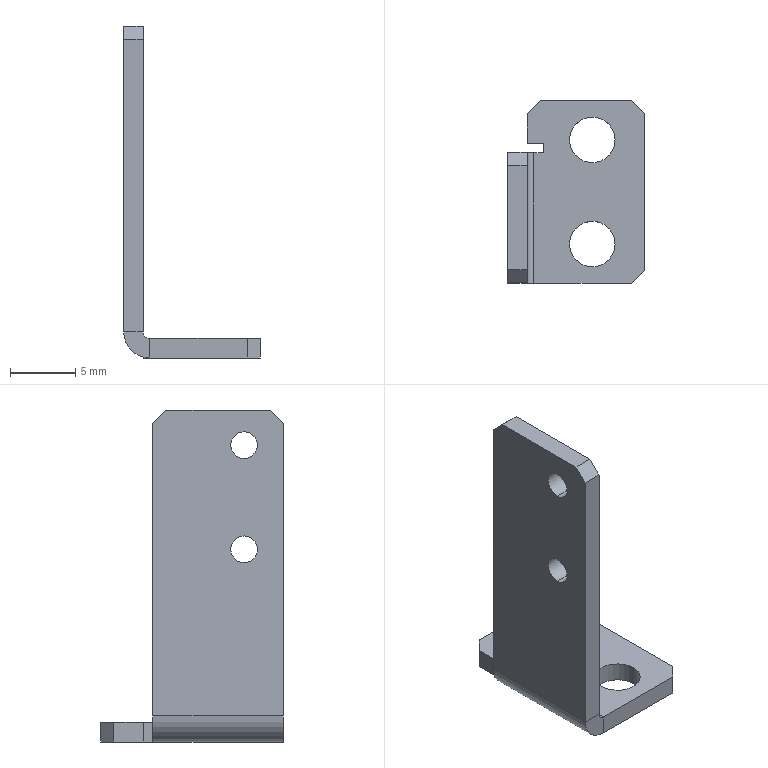Part | SolidWorks | features HoleWzd 2, Chamfer 1, EdgeFlange 1, FlatPattern 1, SMBaseFlange 1, SheetMetal 1 | 1 solid | 31 faces | box 10.5 x 14 x 25.5 mm | volume 519.531 mm3 | plane 21 | cylinder 10 | commonest cylinder face diameters 2.05 x4 3.5 x4 1 x1 4 x1
STEP:
#1=CARTESIAN_POINT('',(-1.25,-4.,-1.5));
#2=VERTEX_POINT('',#1);
#3=CARTESIAN_POINT('',(2.25,-4.,-1.5));
#4=VERTEX_POINT('',#3);
#5=CARTESIAN_POINT('',(0.5,-4.,-1.5));
#6=DIRECTION('',(0.,0.,1.));
#7=DIRECTION('',(1.,0.,0.));
#8=AXIS2_PLACEMENT_3D('',#5,#6,#7);
#9=CIRCLE('',#8,1.75);
#10=EDGE_CURVE('',#2,#4,#9,.T.);
#11=ORIENTED_EDGE('',*,*,#10,.F.);
#12=CARTESIAN_POINT('',(-1.25,-4.,0.));
#13=VERTEX_POINT('',#12);
#14=CARTESIAN_POINT('',(-1.25,-4.,0.));
#15=DIRECTION('',(0.,0.,1.));
#16=VECTOR('',#15,1000.);
#17=LINE('',#14,#16);
#18=EDGE_CURVE('',#2,#13,#17,.T.);
#19=ORIENTED_EDGE('',*,*,#18,.T.);
#20=CARTESIAN_POINT('',(2.25,-4.,0.));
#21=VERTEX_POINT('',#20);
#22=CARTESIAN_POINT('',(0.5,-4.,0.));
#23=DIRECTION('',(0.,0.,1.));
#24=DIRECTION('',(1.,0.,0.));
#25=AXIS2_PLACEMENT_3D('',#22,#23,#24);
#26=CIRCLE('',#25,1.75);
#27=EDGE_CURVE('',#13,#21,#26,.T.);
#28=ORIENTED_EDGE('',*,*,#27,.T.);
#29=CARTESIAN_POINT('',(2.25,-4.,0.));
#30=DIRECTION('',(0.,0.,1.));
#31=VECTOR('',#30,1000.);
#32=LINE('',#29,#31);
#33=EDGE_CURVE('',#4,#21,#32,.T.);
#34=ORIENTED_EDGE('',*,*,#33,.F.);
#35=EDGE_LOOP('',(#11,#19,#28,#34));
#36=FACE_OUTER_BOUND('',#35,.T.);
#37=CARTESIAN_POINT('',(0.5,-4.,0.));
#38=DIRECTION('',(0.,0.,1.));
#39=DIRECTION('',(1.,0.,0.));
#40=AXIS2_PLACEMENT_3D('',#37,#38,#39);
#41=CYLINDRICAL_SURFACE('',#40,1.75);
#42=ADVANCED_FACE('',(#36),#41,.F.);
#43=CARTESIAN_POINT('',(-1.25,4.,-1.5));
#44=VERTEX_POINT('',#43);
#45=CARTESIAN_POINT('',(2.25,4.,-1.5));
#46=VERTEX_POINT('',#45);
#47=CARTESIAN_POINT('',(0.5,4.,-1.5));
#48=DIRECTION('',(0.,0.,1.));
#49=DIRECTION('',(1.,0.,0.));
#50=AXIS2_PLACEMENT_3D('',#47,#48,#49);
#51=CIRCLE('',#50,1.75);
#52=EDGE_CURVE('',#44,#46,#51,.T.);
#53=ORIENTED_EDGE('',*,*,#52,.F.);
#54=CARTESIAN_POINT('',(-1.25,4.,0.));
#55=VERTEX_POINT('',#54);
#56=CARTESIAN_POINT('',(-1.25,4.,0.));
#57=DIRECTION('',(0.,0.,1.));
#58=VECTOR('',#57,1000.);
#59=LINE('',#56,#58);
#60=EDGE_CURVE('',#44,#55,#59,.T.);
#61=ORIENTED_EDGE('',*,*,#60,.T.);
#62=CARTESIAN_POINT('',(2.25,4.,0.));
#63=VERTEX_POINT('',#62);
#64=CARTESIAN_POINT('',(0.5,4.,0.));
#65=DIRECTION('',(0.,0.,1.));
#66=DIRECTION('',(1.,0.,0.));
#67=AXIS2_PLACEMENT_3D('',#64,#65,#66);
#68=CIRCLE('',#67,1.75);
#69=EDGE_CURVE('',#55,#63,#68,.T.);
#70=ORIENTED_EDGE('',*,*,#69,.T.);
#71=CARTESIAN_POINT('',(2.25,4.,0.));
#72=DIRECTION('',(0.,0.,1.));
#73=VECTOR('',#72,1000.);
#74=LINE('',#71,#73);
#75=EDGE_CURVE('',#46,#63,#74,.T.);
#76=ORIENTED_EDGE('',*,*,#75,.F.);
#77=EDGE_LOOP('',(#53,#61,#70,#76));
#78=FACE_OUTER_BOUND('',#77,.T.);
#79=CARTESIAN_POINT('',(0.5,4.,0.));
#80=DIRECTION('',(0.,0.,1.));
#81=DIRECTION('',(1.,0.,0.));
#82=AXIS2_PLACEMENT_3D('',#79,#80,#81);
#83=CYLINDRICAL_SURFACE('',#82,1.75);
#84=ADVANCED_FACE('',(#78),#83,.F.);
#85=CARTESIAN_POINT('',(-4.5,-4.,14.325));
#86=VERTEX_POINT('',#85);
#87=CARTESIAN_POINT('',(-4.5,-4.,12.275));
#88=VERTEX_POINT('',#87);
#89=CARTESIAN_POINT('',(-4.5,-4.,13.3));
#90=DIRECTION('',(1.,0.,0.));
#91=DIRECTION('',(0.,0.,-1.));
#92=AXIS2_PLACEMENT_3D('',#89,#90,#91);
#93=CIRCLE('',#92,1.025);
#94=EDGE_CURVE('',#86,#88,#93,.T.);
#95=ORIENTED_EDGE('',*,*,#94,.T.);
#96=CARTESIAN_POINT('',(-6.,-4.,12.275));
#97=VERTEX_POINT('',#96);
#98=CARTESIAN_POINT('',(-6.,-4.,12.275));
#99=DIRECTION('',(-1.,0.,0.));
#100=VECTOR('',#99,1000.);
#101=LINE('',#98,#100);
#102=EDGE_CURVE('',#88,#97,#101,.T.);
#103=ORIENTED_EDGE('',*,*,#102,.T.);
#104=CARTESIAN_POINT('',(-6.,-4.,14.325));
#105=VERTEX_POINT('',#104);
#106=CARTESIAN_POINT('',(-6.,-4.,13.3));
#107=DIRECTION('',(-1.,0.,0.));
#108=DIRECTION('',(0.,0.,1.));
#109=AXIS2_PLACEMENT_3D('',#106,#107,#108);
#110=CIRCLE('',#109,1.025);
#111=EDGE_CURVE('',#97,#105,#110,.T.);
#112=ORIENTED_EDGE('',*,*,#111,.T.);
#113=CARTESIAN_POINT('',(-6.,-4.,14.325));
#114=DIRECTION('',(-1.,0.,0.));
#115=VECTOR('',#114,1000.);
#116=LINE('',#113,#115);
#117=EDGE_CURVE('',#86,#105,#116,.T.);
#118=ORIENTED_EDGE('',*,*,#117,.F.);
#119=EDGE_LOOP('',(#95,#103,#112,#118));
#120=FACE_OUTER_BOUND('',#119,.T.);
#121=CARTESIAN_POINT('',(-6.,-4.,13.3));
#122=DIRECTION('',(-1.,0.,0.));
#123=DIRECTION('',(0.,0.,1.));
#124=AXIS2_PLACEMENT_3D('',#121,#122,#123);
#125=CYLINDRICAL_SURFACE('',#124,1.025);
#126=ADVANCED_FACE('',(#120),#125,.F.);
#127=CARTESIAN_POINT('',(-4.5,-4.,22.325));
#128=VERTEX_POINT('',#127);
#129=CARTESIAN_POINT('',(-4.5,-4.,20.275));
#130=VERTEX_POINT('',#129);
#131=CARTESIAN_POINT('',(-4.5,-4.,21.3));
#132=DIRECTION('',(1.,0.,0.));
#133=DIRECTION('',(0.,0.,-1.));
#134=AXIS2_PLACEMENT_3D('',#131,#132,#133);
#135=CIRCLE('',#134,1.025);
#136=EDGE_CURVE('',#128,#130,#135,.T.);
#137=ORIENTED_EDGE('',*,*,#136,.T.);
#138=CARTESIAN_POINT('',(-6.,-4.,20.275));
#139=VERTEX_POINT('',#138);
#140=CARTESIAN_POINT('',(-6.,-4.,20.275));
#141=DIRECTION('',(-1.,0.,0.));
#142=VECTOR('',#141,1000.);
#143=LINE('',#140,#142);
#144=EDGE_CURVE('',#130,#139,#143,.T.);
#145=ORIENTED_EDGE('',*,*,#144,.T.);
#146=CARTESIAN_POINT('',(-6.,-4.,22.325));
#147=VERTEX_POINT('',#146);
#148=CARTESIAN_POINT('',(-6.,-4.,21.3));
#149=DIRECTION('',(-1.,0.,0.));
#150=DIRECTION('',(0.,0.,1.));
#151=AXIS2_PLACEMENT_3D('',#148,#149,#150);
#152=CIRCLE('',#151,1.025);
#153=EDGE_CURVE('',#139,#147,#152,.T.);
#154=ORIENTED_EDGE('',*,*,#153,.T.);
#155=CARTESIAN_POINT('',(-6.,-4.,22.325));
#156=DIRECTION('',(-1.,0.,0.));
#157=VECTOR('',#156,1000.);
#158=LINE('',#155,#157);
#159=EDGE_CURVE('',#128,#147,#158,.T.);
#160=ORIENTED_EDGE('',*,*,#159,.F.);
#161=EDGE_LOOP('',(#137,#145,#154,#160));
#162=FACE_OUTER_BOUND('',#161,.T.);
#163=CARTESIAN_POINT('',(-6.,-4.,21.3));
#164=DIRECTION('',(-1.,0.,0.));
#165=DIRECTION('',(0.,0.,1.));
#166=AXIS2_PLACEMENT_3D('',#163,#164,#165);
#167=CYLINDRICAL_SURFACE('',#166,1.025);
#168=ADVANCED_FACE('',(#162),#167,.F.);
#169=CARTESIAN_POINT('',(-4.,-7.,-1.5));
#170=VERTEX_POINT('',#169);
#171=CARTESIAN_POINT('',(3.5,-7.,-1.5));
#172=VERTEX_POINT('',#171);
#173=CARTESIAN_POINT('',(-4.5,-7.,-1.5));
#174=DIRECTION('',(1.,0.,0.));
#175=VECTOR('',#174,1000.);
#176=LINE('',#173,#175);
#177=EDGE_CURVE('',#170,#172,#176,.T.);
#178=ORIENTED_EDGE('',*,*,#177,.T.);
#179=CARTESIAN_POINT('',(3.5,-7.,0.));
#180=VERTEX_POINT('',#179);
#181=CARTESIAN_POINT('',(3.5,-7.,-1.5));
#182=DIRECTION('',(0.,0.,1.));
#183=VECTOR('',#182,1000.);
#184=LINE('',#181,#183);
#185=EDGE_CURVE('',#172,#180,#184,.T.);
#186=ORIENTED_EDGE('',*,*,#185,.T.);
#187=CARTESIAN_POINT('',(-4.,-7.,0.));
#188=VERTEX_POINT('',#187);
#189=CARTESIAN_POINT('',(-4.5,-7.,0.));
#190=DIRECTION('',(1.,0.,0.));
#191=VECTOR('',#190,1000.);
#192=LINE('',#189,#191);
#193=EDGE_CURVE('',#188,#180,#192,.T.);
#194=ORIENTED_EDGE('',*,*,#193,.F.);
#195=CARTESIAN_POINT('',(-4.,-7.,0.));
#196=DIRECTION('',(0.,0.,-1.));
#197=VECTOR('',#196,1000.);
#198=LINE('',#195,#197);
#199=EDGE_CURVE('',#188,#170,#198,.T.);
#200=ORIENTED_EDGE('',*,*,#199,.T.);
#201=EDGE_LOOP('',(#178,#186,#194,#200));
#202=FACE_OUTER_BOUND('',#201,.T.);
#203=CARTESIAN_POINT('',(-4.5,-7.,-1.5));
#204=DIRECTION('',(0.,-1.,0.));
#205=DIRECTION('',(0.,0.,-1.));
#206=AXIS2_PLACEMENT_3D('',#203,#204,#205);
#207=PLANE('',#206);
#208=ADVANCED_FACE('',(#202),#207,.T.);
#209=CARTESIAN_POINT('',(-4.5,6.,0.));
#210=VERTEX_POINT('',#209);
#211=CARTESIAN_POINT('',(-4.5,3.75,0.));
#212=VERTEX_POINT('',#211);
#213=CARTESIAN_POINT('',(-4.5,7.,0.));
#214=DIRECTION('',(0.,-1.,0.));
#215=VECTOR('',#214,1000.);
#216=LINE('',#213,#215);
#217=EDGE_CURVE('',#210,#212,#216,.T.);
#218=ORIENTED_EDGE('',*,*,#217,.F.);
#219=CARTESIAN_POINT('',(-4.5,6.,-1.5));
#220=VERTEX_POINT('',#219);
#221=CARTESIAN_POINT('',(-4.5,6.,-1.5));
#222=DIRECTION('',(0.,0.,-1.));
#223=VECTOR('',#222,1000.);
#224=LINE('',#221,#223);
#225=EDGE_CURVE('',#210,#220,#224,.T.);
#226=ORIENTED_EDGE('',*,*,#225,.T.);
#227=CARTESIAN_POINT('',(-4.5,3.75,-1.5));
#228=VERTEX_POINT('',#227);
#229=CARTESIAN_POINT('',(-4.5,7.,-1.5));
#230=DIRECTION('',(0.,-1.,0.));
#231=VECTOR('',#230,1000.);
#232=LINE('',#229,#231);
#233=EDGE_CURVE('',#220,#228,#232,.T.);
#234=ORIENTED_EDGE('',*,*,#233,.T.);
#235=CARTESIAN_POINT('',(-4.5,3.75,0.));
#236=DIRECTION('',(0.,0.,-1.));
#237=VECTOR('',#236,1000.);
#238=LINE('',#235,#237);
#239=EDGE_CURVE('',#212,#228,#238,.T.);
#240=ORIENTED_EDGE('',*,*,#239,.F.);
#241=EDGE_LOOP('',(#218,#226,#234,#240));
#242=FACE_OUTER_BOUND('',#241,.T.);
#243=CARTESIAN_POINT('',(-4.5,7.,-1.5));
#244=DIRECTION('',(-1.,0.,0.));
#245=DIRECTION('',(0.,-1.,0.));
#246=AXIS2_PLACEMENT_3D('',#243,#244,#245);
#247=PLANE('',#246);
#248=ADVANCED_FACE('',(#242),#247,.T.);
#249=CARTESIAN_POINT('',(0.5,-4.,-1.5));
#250=DIRECTION('',(0.,0.,1.));
#251=DIRECTION('',(1.,0.,0.));
#252=AXIS2_PLACEMENT_3D('',#249,#250,#251);
#253=CIRCLE('',#252,1.75);
#254=EDGE_CURVE('',#4,#2,#253,.T.);
#255=ORIENTED_EDGE('',*,*,#254,.T.);
#256=ORIENTED_EDGE('',*,*,#10,.T.);
#257=EDGE_LOOP('',(#255,#256));
#258=FACE_BOUND('',#257,.T.);
#259=CARTESIAN_POINT('',(0.5,4.,-1.5));
#260=DIRECTION('',(0.,0.,1.));
#261=DIRECTION('',(1.,0.,0.));
#262=AXIS2_PLACEMENT_3D('',#259,#260,#261);
#263=CIRCLE('',#262,1.75);
#264=EDGE_CURVE('',#46,#44,#263,.T.);
#265=ORIENTED_EDGE('',*,*,#264,.T.);
#266=ORIENTED_EDGE('',*,*,#52,.T.);
#267=EDGE_LOOP('',(#265,#266));
#268=FACE_BOUND('',#267,.T.);
#269=ORIENTED_EDGE('',*,*,#233,.F.);
#270=CARTESIAN_POINT('',(-3.5,7.,-1.5));
#271=VERTEX_POINT('',#270);
#272=CARTESIAN_POINT('',(-3.5,7.,-1.5));
#273=DIRECTION('',(0.7071,0.7071,0.));
#274=VECTOR('',#273,1000.);
#275=LINE('',#272,#274);
#276=EDGE_CURVE('',#220,#271,#275,.T.);
#277=ORIENTED_EDGE('',*,*,#276,.T.);
#278=CARTESIAN_POINT('',(3.5,7.,-1.5));
#279=VERTEX_POINT('',#278);
#280=CARTESIAN_POINT('',(-4.5,7.,-1.5));
#281=DIRECTION('',(-1.,0.,0.));
#282=VECTOR('',#281,1000.);
#283=LINE('',#280,#282);
#284=EDGE_CURVE('',#279,#271,#283,.T.);
#285=ORIENTED_EDGE('',*,*,#284,.F.);
#286=CARTESIAN_POINT('',(4.5,6.,-1.5));
#287=VERTEX_POINT('',#286);
#288=CARTESIAN_POINT('',(4.5,6.,-1.5));
#289=DIRECTION('',(0.7071,-0.7071,0.));
#290=VECTOR('',#289,1000.);
#291=LINE('',#288,#290);
#292=EDGE_CURVE('',#279,#287,#291,.T.);
#293=ORIENTED_EDGE('',*,*,#292,.T.);
#294=CARTESIAN_POINT('',(4.5,-6.,-1.5));
#295=VERTEX_POINT('',#294);
#296=CARTESIAN_POINT('',(4.5,7.,-1.5));
#297=DIRECTION('',(0.,1.,0.));
#298=VECTOR('',#297,1000.);
#299=LINE('',#296,#298);
#300=EDGE_CURVE('',#295,#287,#299,.T.);
#301=ORIENTED_EDGE('',*,*,#300,.F.);
#302=CARTESIAN_POINT('',(3.5,-7.,-1.5));
#303=DIRECTION('',(-0.7071,-0.7071,0.));
#304=VECTOR('',#303,1000.);
#305=LINE('',#302,#304);
#306=EDGE_CURVE('',#295,#172,#305,.T.);
#307=ORIENTED_EDGE('',*,*,#306,.T.);
#308=ORIENTED_EDGE('',*,*,#177,.F.);
#309=CARTESIAN_POINT('',(-4.,3.,-1.5));
#310=VERTEX_POINT('',#309);
#311=CARTESIAN_POINT('',(-4.,-7.,-1.5));
#312=DIRECTION('',(0.,1.,0.));
#313=VECTOR('',#312,1000.);
#314=LINE('',#311,#313);
#315=EDGE_CURVE('',#170,#310,#314,.T.);
#316=ORIENTED_EDGE('',*,*,#315,.T.);
#317=CARTESIAN_POINT('',(-3.25,3.,-1.5));
#318=VERTEX_POINT('',#317);
#319=CARTESIAN_POINT('',(0.,3.,-1.5));
#320=DIRECTION('',(-1.,0.,0.));
#321=VECTOR('',#320,1000.);
#322=LINE('',#319,#321);
#323=EDGE_CURVE('',#318,#310,#322,.T.);
#324=ORIENTED_EDGE('',*,*,#323,.F.);
#325=CARTESIAN_POINT('',(-3.25,3.75,-1.5));
#326=VERTEX_POINT('',#325);
#327=CARTESIAN_POINT('',(-3.25,0.,-1.5));
#328=DIRECTION('',(0.,-1.,0.));
#329=VECTOR('',#328,1000.);
#330=LINE('',#327,#329);
#331=EDGE_CURVE('',#326,#318,#330,.T.);
#332=ORIENTED_EDGE('',*,*,#331,.F.);
#333=CARTESIAN_POINT('',(0.,3.75,-1.5));
#334=DIRECTION('',(1.,0.,0.));
#335=VECTOR('',#334,1000.);
#336=LINE('',#333,#335);
#337=EDGE_CURVE('',#228,#326,#336,.T.);
#338=ORIENTED_EDGE('',*,*,#337,.F.);
#339=EDGE_LOOP('',(#269,#277,#285,#293,#301,#307,#308,#316,#324,#332,#338));
#340=FACE_OUTER_BOUND('',#339,.T.);
#341=CARTESIAN_POINT('',(0.,0.,-1.5));
#342=DIRECTION('',(0.,0.,1.));
#343=DIRECTION('',(1.,0.,0.));
#344=AXIS2_PLACEMENT_3D('',#341,#342,#343);
#345=PLANE('',#344);
#346=ADVANCED_FACE('',(#258,#268,#340),#345,.F.);
#347=CARTESIAN_POINT('',(0.5,-4.,0.));
#348=DIRECTION('',(0.,0.,1.));
#349=DIRECTION('',(1.,0.,0.));
#350=AXIS2_PLACEMENT_3D('',#347,#348,#349);
#351=CIRCLE('',#350,1.75);
#352=EDGE_CURVE('',#21,#13,#351,.T.);
#353=ORIENTED_EDGE('',*,*,#352,.F.);
#354=ORIENTED_EDGE('',*,*,#27,.F.);
#355=EDGE_LOOP('',(#353,#354));
#356=FACE_BOUND('',#355,.T.);
#357=CARTESIAN_POINT('',(0.5,4.,0.));
#358=DIRECTION('',(0.,0.,1.));
#359=DIRECTION('',(1.,0.,0.));
#360=AXIS2_PLACEMENT_3D('',#357,#358,#359);
#361=CIRCLE('',#360,1.75);
#362=EDGE_CURVE('',#63,#55,#361,.T.);
#363=ORIENTED_EDGE('',*,*,#362,.F.);
#364=ORIENTED_EDGE('',*,*,#69,.F.);
#365=EDGE_LOOP('',(#363,#364));
#366=FACE_BOUND('',#365,.T.);
#367=CARTESIAN_POINT('',(3.5,7.,0.));
#368=VERTEX_POINT('',#367);
#369=CARTESIAN_POINT('',(-3.5,7.,0.));
#370=VERTEX_POINT('',#369);
#371=CARTESIAN_POINT('',(-4.5,7.,0.));
#372=DIRECTION('',(-1.,0.,0.));
#373=VECTOR('',#372,1000.);
#374=LINE('',#371,#373);
#375=EDGE_CURVE('',#368,#370,#374,.T.);
#376=ORIENTED_EDGE('',*,*,#375,.T.);
#377=CARTESIAN_POINT('',(-5.25,5.25,0.));
#378=DIRECTION('',(-0.7071,-0.7071,0.));
#379=VECTOR('',#378,1000.);
#380=LINE('',#377,#379);
#381=EDGE_CURVE('',#370,#210,#380,.T.);
#382=ORIENTED_EDGE('',*,*,#381,.T.);
#383=ORIENTED_EDGE('',*,*,#217,.T.);
#384=CARTESIAN_POINT('',(-3.25,3.75,0.));
#385=VERTEX_POINT('',#384);
#386=CARTESIAN_POINT('',(-3.25,3.75,0.));
#387=DIRECTION('',(-1.,0.,0.));
#388=VECTOR('',#387,1000.);
#389=LINE('',#386,#388);
#390=EDGE_CURVE('',#385,#212,#389,.T.);
#391=ORIENTED_EDGE('',*,*,#390,.F.);
#392=CARTESIAN_POINT('',(-3.25,3.,0.));
#393=VERTEX_POINT('',#392);
#394=CARTESIAN_POINT('',(-3.25,3.,0.));
#395=DIRECTION('',(0.,1.,0.));
#396=VECTOR('',#395,1000.);
#397=LINE('',#394,#396);
#398=EDGE_CURVE('',#393,#385,#397,.T.);
#399=ORIENTED_EDGE('',*,*,#398,.F.);
#400=CARTESIAN_POINT('',(-4.,3.,0.));
#401=VERTEX_POINT('',#400);
#402=CARTESIAN_POINT('',(-4.,3.,0.));
#403=DIRECTION('',(1.,0.,0.));
#404=VECTOR('',#403,1000.);
#405=LINE('',#402,#404);
#406=EDGE_CURVE('',#401,#393,#405,.T.);
#407=ORIENTED_EDGE('',*,*,#406,.F.);
#408=CARTESIAN_POINT('',(-4.,-7.,0.));
#409=DIRECTION('',(0.,1.,0.));
#410=VECTOR('',#409,1000.);
#411=LINE('',#408,#410);
#412=EDGE_CURVE('',#188,#401,#411,.T.);
#413=ORIENTED_EDGE('',*,*,#412,.F.);
#414=ORIENTED_EDGE('',*,*,#193,.T.);
#415=CARTESIAN_POINT('',(4.5,-6.,0.));
#416=VERTEX_POINT('',#415);
#417=CARTESIAN_POINT('',(5.25,-5.25,0.));
#418=DIRECTION('',(0.7071,0.7071,0.));
#419=VECTOR('',#418,1000.);
#420=LINE('',#417,#419);
#421=EDGE_CURVE('',#180,#416,#420,.T.);
#422=ORIENTED_EDGE('',*,*,#421,.T.);
#423=CARTESIAN_POINT('',(4.5,6.,0.));
#424=VERTEX_POINT('',#423);
#425=CARTESIAN_POINT('',(4.5,7.,0.));
#426=DIRECTION('',(0.,1.,0.));
#427=VECTOR('',#426,1000.);
#428=LINE('',#425,#427);
#429=EDGE_CURVE('',#416,#424,#428,.T.);
#430=ORIENTED_EDGE('',*,*,#429,.T.);
#431=CARTESIAN_POINT('',(5.25,5.25,0.));
#432=DIRECTION('',(-0.7071,0.7071,0.));
#433=VECTOR('',#432,1000.);
#434=LINE('',#431,#433);
#435=EDGE_CURVE('',#424,#368,#434,.T.);
#436=ORIENTED_EDGE('',*,*,#435,.T.);
#437=EDGE_LOOP('',(#376,#382,#383,#391,#399,#407,#413,#414,#422,#430,#436));
#438=FACE_OUTER_BOUND('',#437,.T.);
#439=CARTESIAN_POINT('',(0.,0.,0.));
#440=DIRECTION('',(0.,0.,1.));
#441=DIRECTION('',(1.,0.,0.));
#442=AXIS2_PLACEMENT_3D('',#439,#440,#441);
#443=PLANE('',#442);
#444=ADVANCED_FACE('',(#356,#366,#438),#443,.T.);
#445=ORIENTED_EDGE('',*,*,#300,.T.);
#446=CARTESIAN_POINT('',(4.5,6.,-1.5));
#447=DIRECTION('',(0.,0.,1.));
#448=VECTOR('',#447,1000.);
#449=LINE('',#446,#448);
#450=EDGE_CURVE('',#287,#424,#449,.T.);
#451=ORIENTED_EDGE('',*,*,#450,.T.);
#452=ORIENTED_EDGE('',*,*,#429,.F.);
#453=CARTESIAN_POINT('',(4.5,-6.,-1.5));
#454=DIRECTION('',(0.,0.,-1.));
#455=VECTOR('',#454,1000.);
#456=LINE('',#453,#455);
#457=EDGE_CURVE('',#416,#295,#456,.T.);
#458=ORIENTED_EDGE('',*,*,#457,.T.);
#459=EDGE_LOOP('',(#445,#451,#452,#458));
#460=FACE_OUTER_BOUND('',#459,.T.);
#461=CARTESIAN_POINT('',(4.5,7.,-1.5));
#462=DIRECTION('',(1.,0.,0.));
#463=DIRECTION('',(0.,1.,0.));
#464=AXIS2_PLACEMENT_3D('',#461,#462,#463);
#465=PLANE('',#464);
#466=ADVANCED_FACE('',(#460),#465,.T.);
#467=ORIENTED_EDGE('',*,*,#284,.T.);
#468=CARTESIAN_POINT('',(-3.5,7.,-1.5));
#469=DIRECTION('',(0.,0.,1.));
#470=VECTOR('',#469,1000.);
#471=LINE('',#468,#470);
#472=EDGE_CURVE('',#271,#370,#471,.T.);
#473=ORIENTED_EDGE('',*,*,#472,.T.);
#474=ORIENTED_EDGE('',*,*,#375,.F.);
#475=CARTESIAN_POINT('',(3.5,7.,-1.5));
#476=DIRECTION('',(0.,0.,-1.));
#477=VECTOR('',#476,1000.);
#478=LINE('',#475,#477);
#479=EDGE_CURVE('',#368,#279,#478,.T.);
#480=ORIENTED_EDGE('',*,*,#479,.T.);
#481=EDGE_LOOP('',(#467,#473,#474,#480));
#482=FACE_OUTER_BOUND('',#481,.T.);
#483=CARTESIAN_POINT('',(-4.5,7.,-1.5));
#484=DIRECTION('',(0.,1.,0.));
#485=DIRECTION('',(0.,0.,1.));
#486=AXIS2_PLACEMENT_3D('',#483,#484,#485);
#487=PLANE('',#486);
#488=ADVANCED_FACE('',(#482),#487,.T.);
#489=CARTESIAN_POINT('',(-3.25,3.,0.));
#490=DIRECTION('',(0.,0.,-1.));
#491=VECTOR('',#490,1000.);
#492=LINE('',#489,#491);
#493=EDGE_CURVE('',#393,#318,#492,.T.);
#494=ORIENTED_EDGE('',*,*,#493,.T.);
#495=ORIENTED_EDGE('',*,*,#323,.T.);
#496=CARTESIAN_POINT('',(-4.,3.,0.));
#497=DIRECTION('',(0.,0.,-1.));
#498=VECTOR('',#497,1000.);
#499=LINE('',#496,#498);
#500=EDGE_CURVE('',#401,#310,#499,.T.);
#501=ORIENTED_EDGE('',*,*,#500,.F.);
#502=ORIENTED_EDGE('',*,*,#406,.T.);
#503=EDGE_LOOP('',(#494,#495,#501,#502));
#504=FACE_OUTER_BOUND('',#503,.T.);
#505=CARTESIAN_POINT('',(-4.,3.,0.));
#506=DIRECTION('',(0.,1.,0.));
#507=DIRECTION('',(0.,0.,1.));
#508=AXIS2_PLACEMENT_3D('',#505,#506,#507);
#509=PLANE('',#508);
#510=ADVANCED_FACE('',(#504),#509,.T.);
#511=CARTESIAN_POINT('',(-3.25,3.75,0.));
#512=DIRECTION('',(0.,0.,-1.));
#513=VECTOR('',#512,1000.);
#514=LINE('',#511,#513);
#515=EDGE_CURVE('',#385,#326,#514,.T.);
#516=ORIENTED_EDGE('',*,*,#515,.T.);
#517=ORIENTED_EDGE('',*,*,#331,.T.);
#518=ORIENTED_EDGE('',*,*,#493,.F.);
#519=ORIENTED_EDGE('',*,*,#398,.T.);
#520=EDGE_LOOP('',(#516,#517,#518,#519));
#521=FACE_OUTER_BOUND('',#520,.T.);
#522=CARTESIAN_POINT('',(-3.25,3.,0.));
#523=DIRECTION('',(-1.,0.,0.));
#524=DIRECTION('',(0.,0.,1.));
#525=AXIS2_PLACEMENT_3D('',#522,#523,#524);
#526=PLANE('',#525);
#527=ADVANCED_FACE('',(#521),#526,.T.);
#528=ORIENTED_EDGE('',*,*,#239,.T.);
#529=ORIENTED_EDGE('',*,*,#337,.T.);
#530=ORIENTED_EDGE('',*,*,#515,.F.);
#531=ORIENTED_EDGE('',*,*,#390,.T.);
#532=EDGE_LOOP('',(#528,#529,#530,#531));
#533=FACE_OUTER_BOUND('',#532,.T.);
#534=CARTESIAN_POINT('',(-3.25,3.75,0.));
#535=DIRECTION('',(0.,-1.,0.));
#536=DIRECTION('',(0.,0.,-1.));
#537=AXIS2_PLACEMENT_3D('',#534,#535,#536);
#538=PLANE('',#537);
#539=ADVANCED_FACE('',(#533),#538,.T.);
#540=CARTESIAN_POINT('',(-4.5,3.,0.5));
#541=VERTEX_POINT('',#540);
#542=CARTESIAN_POINT('',(-6.,3.,0.5));
#543=VERTEX_POINT('',#542);
#544=CARTESIAN_POINT('',(-4.5,3.,0.5));
#545=DIRECTION('',(-1.,0.,0.));
#546=VECTOR('',#545,1000.);
#547=LINE('',#544,#546);
#548=EDGE_CURVE('',#541,#543,#547,.T.);
#549=ORIENTED_EDGE('',*,*,#548,.F.);
#550=CARTESIAN_POINT('',(-4.,3.,0.5));
#551=DIRECTION('',(0.,1.,0.));
#552=DIRECTION('',(0.,0.,-1.));
#553=AXIS2_PLACEMENT_3D('',#550,#551,#552);
#554=CIRCLE('',#553,0.5);
#555=EDGE_CURVE('',#401,#541,#554,.T.);
#556=ORIENTED_EDGE('',*,*,#555,.F.);
#557=ORIENTED_EDGE('',*,*,#500,.T.);
#558=CARTESIAN_POINT('',(-4.,3.,0.5));
#559=DIRECTION('',(0.,1.,0.));
#560=DIRECTION('',(0.,0.,-1.));
#561=AXIS2_PLACEMENT_3D('',#558,#559,#560);
#562=CIRCLE('',#561,2.);
#563=EDGE_CURVE('',#310,#543,#562,.T.);
#564=ORIENTED_EDGE('',*,*,#563,.T.);
#565=EDGE_LOOP('',(#549,#556,#557,#564));
#566=FACE_OUTER_BOUND('',#565,.T.);
#567=CARTESIAN_POINT('',(-4.,3.,0.5));
#568=DIRECTION('',(0.,1.,0.));
#569=DIRECTION('',(0.,0.,1.));
#570=AXIS2_PLACEMENT_3D('',#567,#568,#569);
#571=PLANE('',#570);
#572=ADVANCED_FACE('',(#566),#571,.T.);
#573=CARTESIAN_POINT('',(-4.5,-7.,0.5));
#574=VERTEX_POINT('',#573);
#575=CARTESIAN_POINT('',(-4.,-7.,0.5));
#576=DIRECTION('',(0.,-1.,0.));
#577=DIRECTION('',(0.,0.,-1.));
#578=AXIS2_PLACEMENT_3D('',#575,#576,#577);
#579=CIRCLE('',#578,0.5);
#580=EDGE_CURVE('',#574,#188,#579,.T.);
#581=ORIENTED_EDGE('',*,*,#580,.F.);
#582=CARTESIAN_POINT('',(-6.,-7.,0.5));
#583=VERTEX_POINT('',#582);
#584=CARTESIAN_POINT('',(-4.5,-7.,0.5));
#585=DIRECTION('',(-1.,0.,0.));
#586=VECTOR('',#585,1000.);
#587=LINE('',#584,#586);
#588=EDGE_CURVE('',#574,#583,#587,.T.);
#589=ORIENTED_EDGE('',*,*,#588,.T.);
#590=CARTESIAN_POINT('',(-4.,-7.,0.5));
#591=DIRECTION('',(0.,-1.,0.));
#592=DIRECTION('',(0.,0.,-1.));
#593=AXIS2_PLACEMENT_3D('',#590,#591,#592);
#594=CIRCLE('',#593,2.);
#595=EDGE_CURVE('',#583,#170,#594,.T.);
#596=ORIENTED_EDGE('',*,*,#595,.T.);
#597=ORIENTED_EDGE('',*,*,#199,.F.);
#598=EDGE_LOOP('',(#581,#589,#596,#597));
#599=FACE_OUTER_BOUND('',#598,.T.);
#600=CARTESIAN_POINT('',(-4.,-7.,0.5));
#601=DIRECTION('',(0.,1.,0.));
#602=DIRECTION('',(0.,0.,1.));
#603=AXIS2_PLACEMENT_3D('',#600,#601,#602);
#604=PLANE('',#603);
#605=ADVANCED_FACE('',(#599),#604,.F.);
#606=ORIENTED_EDGE('',*,*,#315,.F.);
#607=ORIENTED_EDGE('',*,*,#595,.F.);
#608=CARTESIAN_POINT('',(-6.,0.,0.5));
#609=DIRECTION('',(0.,1.,0.));
#610=VECTOR('',#609,1000.);
#611=LINE('',#608,#610);
#612=EDGE_CURVE('',#583,#543,#611,.T.);
#613=ORIENTED_EDGE('',*,*,#612,.T.);
#614=ORIENTED_EDGE('',*,*,#563,.F.);
#615=EDGE_LOOP('',(#606,#607,#613,#614));
#616=FACE_OUTER_BOUND('',#615,.T.);
#617=CARTESIAN_POINT('',(-4.,-7.,0.5));
#618=DIRECTION('',(0.,-1.,0.));
#619=DIRECTION('',(-1.,0.,0.));
#620=AXIS2_PLACEMENT_3D('',#617,#618,#619);
#621=CYLINDRICAL_SURFACE('',#620,2.);
#622=ADVANCED_FACE('',(#616),#621,.T.);
#623=ORIENTED_EDGE('',*,*,#412,.T.);
#624=ORIENTED_EDGE('',*,*,#555,.T.);
#625=CARTESIAN_POINT('',(-4.5,3.,0.5));
#626=DIRECTION('',(0.,-1.,0.));
#627=VECTOR('',#626,1000.);
#628=LINE('',#625,#627);
#629=EDGE_CURVE('',#541,#574,#628,.T.);
#630=ORIENTED_EDGE('',*,*,#629,.T.);
#631=ORIENTED_EDGE('',*,*,#580,.T.);
#632=EDGE_LOOP('',(#623,#624,#630,#631));
#633=FACE_OUTER_BOUND('',#632,.T.);
#634=CARTESIAN_POINT('',(-4.,-7.,0.5));
#635=DIRECTION('',(0.,-1.,0.));
#636=DIRECTION('',(-1.,0.,0.));
#637=AXIS2_PLACEMENT_3D('',#634,#635,#636);
#638=CYLINDRICAL_SURFACE('',#637,0.5);
#639=ADVANCED_FACE('',(#633),#638,.F.);
#640=CARTESIAN_POINT('',(-6.,3.,23.));
#641=VERTEX_POINT('',#640);
#642=CARTESIAN_POINT('',(-6.,3.,0.));
#643=DIRECTION('',(0.,0.,-1.));
#644=VECTOR('',#643,1000.);
#645=LINE('',#642,#644);
#646=EDGE_CURVE('',#641,#543,#645,.T.);
#647=ORIENTED_EDGE('',*,*,#646,.F.);
#648=CARTESIAN_POINT('',(-4.5,3.,23.));
#649=VERTEX_POINT('',#648);
#650=CARTESIAN_POINT('',(-6.,3.,23.));
#651=DIRECTION('',(1.,0.,0.));
#652=VECTOR('',#651,1000.);
#653=LINE('',#650,#652);
#654=EDGE_CURVE('',#641,#649,#653,.T.);
#655=ORIENTED_EDGE('',*,*,#654,.T.);
#656=CARTESIAN_POINT('',(-4.5,3.,0.));
#657=DIRECTION('',(0.,0.,-1.));
#658=VECTOR('',#657,1000.);
#659=LINE('',#656,#658);
#660=EDGE_CURVE('',#649,#541,#659,.T.);
#661=ORIENTED_EDGE('',*,*,#660,.T.);
#662=ORIENTED_EDGE('',*,*,#548,.T.);
#663=EDGE_LOOP('',(#647,#655,#661,#662));
#664=FACE_OUTER_BOUND('',#663,.T.);
#665=CARTESIAN_POINT('',(-6.,3.,0.));
#666=DIRECTION('',(0.,-1.,0.));
#667=DIRECTION('',(1.,0.,0.));
#668=AXIS2_PLACEMENT_3D('',#665,#666,#667);
#669=PLANE('',#668);
#670=ADVANCED_FACE('',(#664),#669,.F.);
#671=CARTESIAN_POINT('',(-4.5,-7.,23.));
#672=VERTEX_POINT('',#671);
#673=CARTESIAN_POINT('',(-4.5,-7.,24.));
#674=DIRECTION('',(0.,0.,1.));
#675=VECTOR('',#674,1000.);
#676=LINE('',#673,#675);
#677=EDGE_CURVE('',#574,#672,#676,.T.);
#678=ORIENTED_EDGE('',*,*,#677,.T.);
#679=CARTESIAN_POINT('',(-6.,-7.,23.));
#680=VERTEX_POINT('',#679);
#681=CARTESIAN_POINT('',(-6.,-7.,23.));
#682=DIRECTION('',(-1.,0.,0.));
#683=VECTOR('',#682,1000.);
#684=LINE('',#681,#683);
#685=EDGE_CURVE('',#672,#680,#684,.T.);
#686=ORIENTED_EDGE('',*,*,#685,.T.);
#687=CARTESIAN_POINT('',(-6.,-7.,24.));
#688=DIRECTION('',(0.,0.,1.));
#689=VECTOR('',#688,1000.);
#690=LINE('',#687,#689);
#691=EDGE_CURVE('',#583,#680,#690,.T.);
#692=ORIENTED_EDGE('',*,*,#691,.F.);
#693=ORIENTED_EDGE('',*,*,#588,.F.);
#694=EDGE_LOOP('',(#678,#686,#692,#693));
#695=FACE_OUTER_BOUND('',#694,.T.);
#696=CARTESIAN_POINT('',(-6.,-7.,24.));
#697=DIRECTION('',(0.,1.,0.));
#698=DIRECTION('',(-1.,0.,0.));
#699=AXIS2_PLACEMENT_3D('',#696,#697,#698);
#700=PLANE('',#699);
#701=ADVANCED_FACE('',(#695),#700,.F.);
#702=CARTESIAN_POINT('',(-6.,-4.,13.3));
#703=DIRECTION('',(-1.,0.,0.));
#704=DIRECTION('',(0.,0.,1.));
#705=AXIS2_PLACEMENT_3D('',#702,#703,#704);
#706=CIRCLE('',#705,1.025);
#707=EDGE_CURVE('',#105,#97,#706,.T.);
#708=ORIENTED_EDGE('',*,*,#707,.F.);
#709=ORIENTED_EDGE('',*,*,#111,.F.);
#710=EDGE_LOOP('',(#708,#709));
#711=FACE_BOUND('',#710,.T.);
#712=CARTESIAN_POINT('',(-6.,-4.,21.3));
#713=DIRECTION('',(-1.,0.,0.));
#714=DIRECTION('',(0.,0.,1.));
#715=AXIS2_PLACEMENT_3D('',#712,#713,#714);
#716=CIRCLE('',#715,1.025);
#717=EDGE_CURVE('',#147,#139,#716,.T.);
#718=ORIENTED_EDGE('',*,*,#717,.F.);
#719=ORIENTED_EDGE('',*,*,#153,.F.);
#720=EDGE_LOOP('',(#718,#719));
#721=FACE_BOUND('',#720,.T.);
#722=ORIENTED_EDGE('',*,*,#691,.T.);
#723=CARTESIAN_POINT('',(-6.,-6.,24.));
#724=VERTEX_POINT('',#723);
#725=CARTESIAN_POINT('',(-6.,-6.,24.));
#726=DIRECTION('',(0.,0.7071,0.7071));
#727=VECTOR('',#726,1000.);
#728=LINE('',#725,#727);
#729=EDGE_CURVE('',#680,#724,#728,.T.);
#730=ORIENTED_EDGE('',*,*,#729,.T.);
#731=CARTESIAN_POINT('',(-6.,2.,24.));
#732=VERTEX_POINT('',#731);
#733=CARTESIAN_POINT('',(-6.,3.,24.));
#734=DIRECTION('',(0.,1.,0.));
#735=VECTOR('',#734,1000.);
#736=LINE('',#733,#735);
#737=EDGE_CURVE('',#724,#732,#736,.T.);
#738=ORIENTED_EDGE('',*,*,#737,.T.);
#739=CARTESIAN_POINT('',(-6.,3.,23.));
#740=DIRECTION('',(0.,0.7071,-0.7071));
#741=VECTOR('',#740,1000.);
#742=LINE('',#739,#741);
#743=EDGE_CURVE('',#732,#641,#742,.T.);
#744=ORIENTED_EDGE('',*,*,#743,.T.);
#745=ORIENTED_EDGE('',*,*,#646,.T.);
#746=ORIENTED_EDGE('',*,*,#612,.F.);
#747=EDGE_LOOP('',(#722,#730,#738,#744,#745,#746));
#748=FACE_OUTER_BOUND('',#747,.T.);
#749=CARTESIAN_POINT('',(-6.,0.,0.));
#750=DIRECTION('',(1.,0.,0.));
#751=DIRECTION('',(0.,0.,-1.));
#752=AXIS2_PLACEMENT_3D('',#749,#750,#751);
#753=PLANE('',#752);
#754=ADVANCED_FACE('',(#711,#721,#748),#753,.F.);
#755=ORIENTED_EDGE('',*,*,#94,.F.);
#756=CARTESIAN_POINT('',(-4.5,-4.,13.3));
#757=DIRECTION('',(1.,0.,0.));
#758=DIRECTION('',(0.,0.,-1.));
#759=AXIS2_PLACEMENT_3D('',#756,#757,#758);
#760=CIRCLE('',#759,1.025);
#761=EDGE_CURVE('',#88,#86,#760,.T.);
#762=ORIENTED_EDGE('',*,*,#761,.F.);
#763=EDGE_LOOP('',(#755,#762));
#764=FACE_BOUND('',#763,.T.);
#765=ORIENTED_EDGE('',*,*,#136,.F.);
#766=CARTESIAN_POINT('',(-4.5,-4.,21.3));
#767=DIRECTION('',(1.,0.,0.));
#768=DIRECTION('',(0.,0.,-1.));
#769=AXIS2_PLACEMENT_3D('',#766,#767,#768);
#770=CIRCLE('',#769,1.025);
#771=EDGE_CURVE('',#130,#128,#770,.T.);
#772=ORIENTED_EDGE('',*,*,#771,.F.);
#773=EDGE_LOOP('',(#765,#772));
#774=FACE_BOUND('',#773,.T.);
#775=CARTESIAN_POINT('',(-4.5,-6.,24.));
#776=VERTEX_POINT('',#775);
#777=CARTESIAN_POINT('',(-4.5,2.,24.));
#778=VERTEX_POINT('',#777);
#779=CARTESIAN_POINT('',(-4.5,3.,24.));
#780=DIRECTION('',(0.,1.,0.));
#781=VECTOR('',#780,1000.);
#782=LINE('',#779,#781);
#783=EDGE_CURVE('',#776,#778,#782,.T.);
#784=ORIENTED_EDGE('',*,*,#783,.F.);
#785=CARTESIAN_POINT('',(-4.5,-15.,15.));
#786=DIRECTION('',(0.,-0.7071,-0.7071));
#787=VECTOR('',#786,1000.);
#788=LINE('',#785,#787);
#789=EDGE_CURVE('',#776,#672,#788,.T.);
#790=ORIENTED_EDGE('',*,*,#789,.T.);
#791=ORIENTED_EDGE('',*,*,#677,.F.);
#792=ORIENTED_EDGE('',*,*,#629,.F.);
#793=ORIENTED_EDGE('',*,*,#660,.F.);
#794=CARTESIAN_POINT('',(-4.5,13.,13.));
#795=DIRECTION('',(0.,-0.7071,0.7071));
#796=VECTOR('',#795,1000.);
#797=LINE('',#794,#796);
#798=EDGE_CURVE('',#649,#778,#797,.T.);
#799=ORIENTED_EDGE('',*,*,#798,.T.);
#800=EDGE_LOOP('',(#784,#790,#791,#792,#793,#799));
#801=FACE_OUTER_BOUND('',#800,.T.);
#802=CARTESIAN_POINT('',(-4.5,0.,0.));
#803=DIRECTION('',(1.,0.,0.));
#804=DIRECTION('',(0.,0.,-1.));
#805=AXIS2_PLACEMENT_3D('',#802,#803,#804);
#806=PLANE('',#805);
#807=ADVANCED_FACE('',(#764,#774,#801),#806,.T.);
#808=ORIENTED_EDGE('',*,*,#737,.F.);
#809=CARTESIAN_POINT('',(-6.,-6.,24.));
#810=DIRECTION('',(1.,0.,0.));
#811=VECTOR('',#810,1000.);
#812=LINE('',#809,#811);
#813=EDGE_CURVE('',#724,#776,#812,.T.);
#814=ORIENTED_EDGE('',*,*,#813,.T.);
#815=ORIENTED_EDGE('',*,*,#783,.T.);
#816=CARTESIAN_POINT('',(-6.,2.,24.));
#817=DIRECTION('',(-1.,0.,0.));
#818=VECTOR('',#817,1000.);
#819=LINE('',#816,#818);
#820=EDGE_CURVE('',#778,#732,#819,.T.);
#821=ORIENTED_EDGE('',*,*,#820,.T.);
#822=EDGE_LOOP('',(#808,#814,#815,#821));
#823=FACE_OUTER_BOUND('',#822,.T.);
#824=CARTESIAN_POINT('',(-6.,3.,24.));
#825=DIRECTION('',(0.,0.,-1.));
#826=DIRECTION('',(-1.,0.,0.));
#827=AXIS2_PLACEMENT_3D('',#824,#825,#826);
#828=PLANE('',#827);
#829=ADVANCED_FACE('',(#823),#828,.F.);
#830=ORIENTED_EDGE('',*,*,#144,.F.);
#831=ORIENTED_EDGE('',*,*,#771,.T.);
#832=ORIENTED_EDGE('',*,*,#159,.T.);
#833=ORIENTED_EDGE('',*,*,#717,.T.);
#834=EDGE_LOOP('',(#830,#831,#832,#833));
#835=FACE_OUTER_BOUND('',#834,.T.);
#836=CARTESIAN_POINT('',(-6.,-4.,21.3));
#837=DIRECTION('',(-1.,0.,0.));
#838=DIRECTION('',(0.,0.,1.));
#839=AXIS2_PLACEMENT_3D('',#836,#837,#838);
#840=CYLINDRICAL_SURFACE('',#839,1.025);
#841=ADVANCED_FACE('',(#835),#840,.F.);
#842=ORIENTED_EDGE('',*,*,#102,.F.);
#843=ORIENTED_EDGE('',*,*,#761,.T.);
#844=ORIENTED_EDGE('',*,*,#117,.T.);
#845=ORIENTED_EDGE('',*,*,#707,.T.);
#846=EDGE_LOOP('',(#842,#843,#844,#845));
#847=FACE_OUTER_BOUND('',#846,.T.);
#848=CARTESIAN_POINT('',(-6.,-4.,13.3));
#849=DIRECTION('',(-1.,0.,0.));
#850=DIRECTION('',(0.,0.,1.));
#851=AXIS2_PLACEMENT_3D('',#848,#849,#850);
#852=CYLINDRICAL_SURFACE('',#851,1.025);
#853=ADVANCED_FACE('',(#847),#852,.F.);
#854=ORIENTED_EDGE('',*,*,#276,.F.);
#855=ORIENTED_EDGE('',*,*,#225,.F.);
#856=ORIENTED_EDGE('',*,*,#381,.F.);
#857=ORIENTED_EDGE('',*,*,#472,.F.);
#858=EDGE_LOOP('',(#854,#855,#856,#857));
#859=FACE_OUTER_BOUND('',#858,.T.);
#860=CARTESIAN_POINT('',(-3.5,7.,-1.5));
#861=DIRECTION('',(0.7071,-0.7071,0.));
#862=DIRECTION('',(0.,0.,1.));
#863=AXIS2_PLACEMENT_3D('',#860,#861,#862);
#864=PLANE('',#863);
#865=ADVANCED_FACE('',(#859),#864,.F.);
#866=ORIENTED_EDGE('',*,*,#292,.F.);
#867=ORIENTED_EDGE('',*,*,#479,.F.);
#868=ORIENTED_EDGE('',*,*,#435,.F.);
#869=ORIENTED_EDGE('',*,*,#450,.F.);
#870=EDGE_LOOP('',(#866,#867,#868,#869));
#871=FACE_OUTER_BOUND('',#870,.T.);
#872=CARTESIAN_POINT('',(4.5,6.,-1.5));
#873=DIRECTION('',(-0.7071,-0.7071,0.));
#874=DIRECTION('',(0.,0.,1.));
#875=AXIS2_PLACEMENT_3D('',#872,#873,#874);
#876=PLANE('',#875);
#877=ADVANCED_FACE('',(#871),#876,.F.);
#878=ORIENTED_EDGE('',*,*,#306,.F.);
#879=ORIENTED_EDGE('',*,*,#457,.F.);
#880=ORIENTED_EDGE('',*,*,#421,.F.);
#881=ORIENTED_EDGE('',*,*,#185,.F.);
#882=EDGE_LOOP('',(#878,#879,#880,#881));
#883=FACE_OUTER_BOUND('',#882,.T.);
#884=CARTESIAN_POINT('',(3.5,-7.,-1.5));
#885=DIRECTION('',(-0.7071,0.7071,0.));
#886=DIRECTION('',(0.,0.,1.));
#887=AXIS2_PLACEMENT_3D('',#884,#885,#886);
#888=PLANE('',#887);
#889=ADVANCED_FACE('',(#883),#888,.F.);
#890=ORIENTED_EDGE('',*,*,#729,.F.);
#891=ORIENTED_EDGE('',*,*,#685,.F.);
#892=ORIENTED_EDGE('',*,*,#789,.F.);
#893=ORIENTED_EDGE('',*,*,#813,.F.);
#894=EDGE_LOOP('',(#890,#891,#892,#893));
#895=FACE_OUTER_BOUND('',#894,.T.);
#896=CARTESIAN_POINT('',(-6.,-6.,24.));
#897=DIRECTION('',(0.,0.7071,-0.7071));
#898=DIRECTION('',(1.,0.,0.));
#899=AXIS2_PLACEMENT_3D('',#896,#897,#898);
#900=PLANE('',#899);
#901=ADVANCED_FACE('',(#895),#900,.F.);
#902=ORIENTED_EDGE('',*,*,#743,.F.);
#903=ORIENTED_EDGE('',*,*,#820,.F.);
#904=ORIENTED_EDGE('',*,*,#798,.F.);
#905=ORIENTED_EDGE('',*,*,#654,.F.);
#906=EDGE_LOOP('',(#902,#903,#904,#905));
#907=FACE_OUTER_BOUND('',#906,.T.);
#908=CARTESIAN_POINT('',(-6.,3.,23.));
#909=DIRECTION('',(0.,-0.7071,-0.7071));
#910=DIRECTION('',(1.,0.,0.));
#911=AXIS2_PLACEMENT_3D('',#908,#909,#910);
#912=PLANE('',#911);
#913=ADVANCED_FACE('',(#907),#912,.F.);
#914=ORIENTED_EDGE('',*,*,#60,.F.);
#915=ORIENTED_EDGE('',*,*,#264,.F.);
#916=ORIENTED_EDGE('',*,*,#75,.T.);
#917=ORIENTED_EDGE('',*,*,#362,.T.);
#918=EDGE_LOOP('',(#914,#915,#916,#917));
#919=FACE_OUTER_BOUND('',#918,.T.);
#920=CARTESIAN_POINT('',(0.5,4.,0.));
#921=DIRECTION('',(0.,0.,1.));
#922=DIRECTION('',(1.,0.,0.));
#923=AXIS2_PLACEMENT_3D('',#920,#921,#922);
#924=CYLINDRICAL_SURFACE('',#923,1.75);
#925=ADVANCED_FACE('',(#919),#924,.F.);
#926=ORIENTED_EDGE('',*,*,#18,.F.);
#927=ORIENTED_EDGE('',*,*,#254,.F.);
#928=ORIENTED_EDGE('',*,*,#33,.T.);
#929=ORIENTED_EDGE('',*,*,#352,.T.);
#930=EDGE_LOOP('',(#926,#927,#928,#929));
#931=FACE_OUTER_BOUND('',#930,.T.);
#932=CARTESIAN_POINT('',(0.5,-4.,0.));
#933=DIRECTION('',(0.,0.,1.));
#934=DIRECTION('',(1.,0.,0.));
#935=AXIS2_PLACEMENT_3D('',#932,#933,#934);
#936=CYLINDRICAL_SURFACE('',#935,1.75);
#937=ADVANCED_FACE('',(#931),#936,.F.);
#938=CLOSED_SHELL('',(#42,#84,#126,#168,#208,#248,#346,#444,#466,#488,#510,#527,#539,#572,#605,#622,#639,#670,#701,#754,#807,#829,#841,#853,#865,#877,#889,#901,#913,#925,#937));
#939=MANIFOLD_SOLID_BREP('',#938);
#940=CARTESIAN_POINT('',(0.,0.,0.));
#941=DIRECTION('',(0.,0.,1.));
#942=DIRECTION('',(1.,0.,0.));
#943=AXIS2_PLACEMENT_3D('',#940,#941,#942);
#944=(LENGTH_UNIT()NAMED_UNIT(*)SI_UNIT(.MILLI.,.METRE.));
#945=UNCERTAINTY_MEASURE_WITH_UNIT(LENGTH_MEASURE(0.00001),#944,'','');
#946=(NAMED_UNIT(*)PLANE_ANGLE_UNIT()SI_UNIT($,.RADIAN.));
#947=(NAMED_UNIT(*)SI_UNIT($,.STERADIAN.)SOLID_ANGLE_UNIT());
#948=(GEOMETRIC_REPRESENTATION_CONTEXT(3)GLOBAL_UNCERTAINTY_ASSIGNED_CONTEXT((#945))GLOBAL_UNIT_ASSIGNED_CONTEXT((#944,#946,#947))REPRESENTATION_CONTEXT('',''));
#949=ADVANCED_BREP_SHAPE_REPRESENTATION('',(#939,#943),#948);